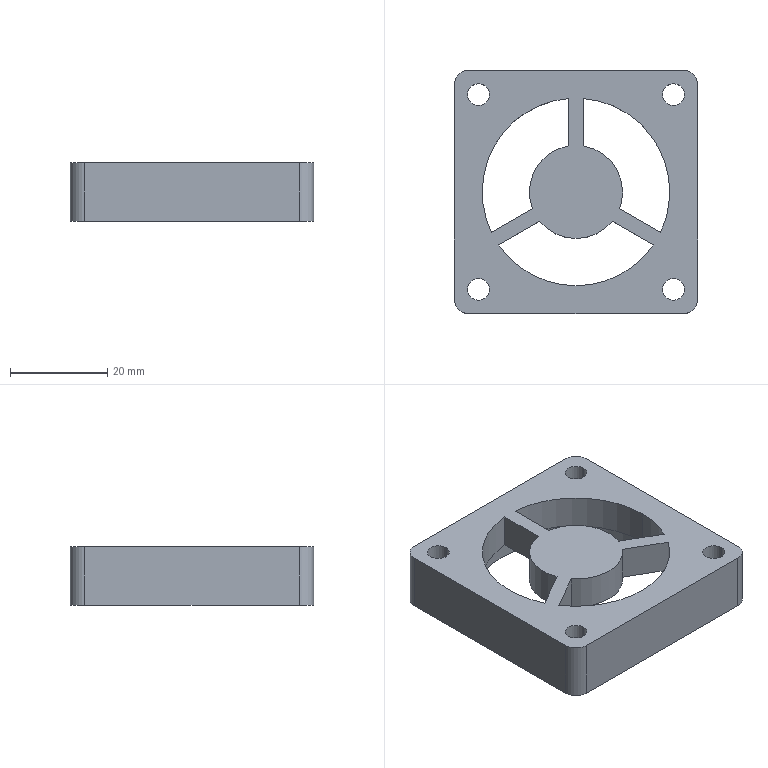Part | SolidWorks | features ICE 2, Extrusion 1 | 1 solid | 35 faces | box 50 x 50 x 12 mm | volume 16391 mm3 | cylinder 22 | plane 13 | commonest cylinder face diameters 4.5 x8 6 x4 19.118 x4 38.495 x4 42.899 x2
STEP:
#1=CARTESIAN_POINT('',(21.45,0.,5.));
#2=VERTEX_POINT('',#1);
#3=CARTESIAN_POINT('',(-21.45,0.,5.));
#4=VERTEX_POINT('',#3);
#5=CARTESIAN_POINT('',(0.,0.,5.));
#6=DIRECTION('',(0.,0.,-1.));
#7=DIRECTION('',(-1.,0.,0.));
#8=AXIS2_PLACEMENT_3D('',#5,#6,#7);
#9=CIRCLE('',#8,21.45);
#10=EDGE_CURVE('',#2,#4,#9,.T.);
#11=ORIENTED_EDGE('',*,*,#10,.F.);
#12=CARTESIAN_POINT('',(21.45,0.,0.));
#13=VERTEX_POINT('',#12);
#14=CARTESIAN_POINT('',(21.45,0.,5.));
#15=DIRECTION('',(0.,0.,-1.));
#16=VECTOR('',#15,1000.);
#17=LINE('',#14,#16);
#18=EDGE_CURVE('',#2,#13,#17,.T.);
#19=ORIENTED_EDGE('',*,*,#18,.T.);
#20=CARTESIAN_POINT('',(-21.45,0.,0.));
#21=VERTEX_POINT('',#20);
#22=CARTESIAN_POINT('',(0.,0.,0.));
#23=DIRECTION('',(0.,0.,-1.));
#24=DIRECTION('',(-1.,0.,0.));
#25=AXIS2_PLACEMENT_3D('',#22,#23,#24);
#26=CIRCLE('',#25,21.45);
#27=EDGE_CURVE('',#13,#21,#26,.T.);
#28=ORIENTED_EDGE('',*,*,#27,.T.);
#29=CARTESIAN_POINT('',(-21.45,0.,5.));
#30=DIRECTION('',(0.,0.,-1.));
#31=VECTOR('',#30,1000.);
#32=LINE('',#29,#31);
#33=EDGE_CURVE('',#4,#21,#32,.T.);
#34=ORIENTED_EDGE('',*,*,#33,.F.);
#35=EDGE_LOOP('',(#11,#19,#28,#34));
#36=FACE_OUTER_BOUND('',#35,.T.);
#37=CARTESIAN_POINT('',(0.,0.,5.));
#38=DIRECTION('',(0.,0.,-1.));
#39=DIRECTION('',(-1.,0.,0.));
#40=AXIS2_PLACEMENT_3D('',#37,#38,#39);
#41=CYLINDRICAL_SURFACE('',#40,21.45);
#42=ADVANCED_FACE('',(#36),#41,.F.);
#43=CARTESIAN_POINT('',(-22.25,-20.,12.));
#44=VERTEX_POINT('',#43);
#45=CARTESIAN_POINT('',(-17.75,-20.,12.));
#46=VERTEX_POINT('',#45);
#47=CARTESIAN_POINT('',(-20.,-20.,12.));
#48=DIRECTION('',(0.,0.,1.));
#49=DIRECTION('',(1.,0.,0.));
#50=AXIS2_PLACEMENT_3D('',#47,#48,#49);
#51=CIRCLE('',#50,2.25);
#52=EDGE_CURVE('',#44,#46,#51,.T.);
#53=ORIENTED_EDGE('',*,*,#52,.T.);
#54=CARTESIAN_POINT('',(-17.75,-20.,0.));
#55=VERTEX_POINT('',#54);
#56=CARTESIAN_POINT('',(-17.75,-20.,12.));
#57=DIRECTION('',(0.,0.,-1.));
#58=VECTOR('',#57,1000.);
#59=LINE('',#56,#58);
#60=EDGE_CURVE('',#46,#55,#59,.T.);
#61=ORIENTED_EDGE('',*,*,#60,.T.);
#62=CARTESIAN_POINT('',(-22.25,-20.,0.));
#63=VERTEX_POINT('',#62);
#64=CARTESIAN_POINT('',(-20.,-20.,0.));
#65=DIRECTION('',(0.,0.,1.));
#66=DIRECTION('',(1.,0.,0.));
#67=AXIS2_PLACEMENT_3D('',#64,#65,#66);
#68=CIRCLE('',#67,2.25);
#69=EDGE_CURVE('',#63,#55,#68,.T.);
#70=ORIENTED_EDGE('',*,*,#69,.F.);
#71=CARTESIAN_POINT('',(-22.25,-20.,12.));
#72=DIRECTION('',(0.,0.,-1.));
#73=VECTOR('',#72,1000.);
#74=LINE('',#71,#73);
#75=EDGE_CURVE('',#44,#63,#74,.T.);
#76=ORIENTED_EDGE('',*,*,#75,.F.);
#77=EDGE_LOOP('',(#53,#61,#70,#76));
#78=FACE_OUTER_BOUND('',#77,.T.);
#79=CARTESIAN_POINT('',(-20.,-20.,12.));
#80=DIRECTION('',(0.,0.,-1.));
#81=DIRECTION('',(-1.,0.,0.));
#82=AXIS2_PLACEMENT_3D('',#79,#80,#81);
#83=CYLINDRICAL_SURFACE('',#82,2.25);
#84=ADVANCED_FACE('',(#78),#83,.F.);
#85=CARTESIAN_POINT('',(17.75,-20.,12.));
#86=VERTEX_POINT('',#85);
#87=CARTESIAN_POINT('',(22.25,-20.,12.));
#88=VERTEX_POINT('',#87);
#89=CARTESIAN_POINT('',(20.,-20.,12.));
#90=DIRECTION('',(0.,0.,1.));
#91=DIRECTION('',(1.,0.,0.));
#92=AXIS2_PLACEMENT_3D('',#89,#90,#91);
#93=CIRCLE('',#92,2.25);
#94=EDGE_CURVE('',#86,#88,#93,.T.);
#95=ORIENTED_EDGE('',*,*,#94,.T.);
#96=CARTESIAN_POINT('',(22.25,-20.,0.));
#97=VERTEX_POINT('',#96);
#98=CARTESIAN_POINT('',(22.25,-20.,12.));
#99=DIRECTION('',(0.,0.,-1.));
#100=VECTOR('',#99,1000.);
#101=LINE('',#98,#100);
#102=EDGE_CURVE('',#88,#97,#101,.T.);
#103=ORIENTED_EDGE('',*,*,#102,.T.);
#104=CARTESIAN_POINT('',(17.75,-20.,0.));
#105=VERTEX_POINT('',#104);
#106=CARTESIAN_POINT('',(20.,-20.,0.));
#107=DIRECTION('',(0.,0.,1.));
#108=DIRECTION('',(1.,0.,0.));
#109=AXIS2_PLACEMENT_3D('',#106,#107,#108);
#110=CIRCLE('',#109,2.25);
#111=EDGE_CURVE('',#105,#97,#110,.T.);
#112=ORIENTED_EDGE('',*,*,#111,.F.);
#113=CARTESIAN_POINT('',(17.75,-20.,12.));
#114=DIRECTION('',(0.,0.,-1.));
#115=VECTOR('',#114,1000.);
#116=LINE('',#113,#115);
#117=EDGE_CURVE('',#86,#105,#116,.T.);
#118=ORIENTED_EDGE('',*,*,#117,.F.);
#119=EDGE_LOOP('',(#95,#103,#112,#118));
#120=FACE_OUTER_BOUND('',#119,.T.);
#121=CARTESIAN_POINT('',(20.,-20.,12.));
#122=DIRECTION('',(0.,0.,-1.));
#123=DIRECTION('',(-1.,0.,0.));
#124=AXIS2_PLACEMENT_3D('',#121,#122,#123);
#125=CYLINDRICAL_SURFACE('',#124,2.25);
#126=ADVANCED_FACE('',(#120),#125,.F.);
#127=CARTESIAN_POINT('',(17.75,20.,12.));
#128=VERTEX_POINT('',#127);
#129=CARTESIAN_POINT('',(22.25,20.,12.));
#130=VERTEX_POINT('',#129);
#131=CARTESIAN_POINT('',(20.,20.,12.));
#132=DIRECTION('',(0.,0.,1.));
#133=DIRECTION('',(1.,0.,0.));
#134=AXIS2_PLACEMENT_3D('',#131,#132,#133);
#135=CIRCLE('',#134,2.25);
#136=EDGE_CURVE('',#128,#130,#135,.T.);
#137=ORIENTED_EDGE('',*,*,#136,.T.);
#138=CARTESIAN_POINT('',(22.25,20.,0.));
#139=VERTEX_POINT('',#138);
#140=CARTESIAN_POINT('',(22.25,20.,12.));
#141=DIRECTION('',(0.,0.,-1.));
#142=VECTOR('',#141,1000.);
#143=LINE('',#140,#142);
#144=EDGE_CURVE('',#130,#139,#143,.T.);
#145=ORIENTED_EDGE('',*,*,#144,.T.);
#146=CARTESIAN_POINT('',(17.75,20.,0.));
#147=VERTEX_POINT('',#146);
#148=CARTESIAN_POINT('',(20.,20.,0.));
#149=DIRECTION('',(0.,0.,1.));
#150=DIRECTION('',(1.,0.,0.));
#151=AXIS2_PLACEMENT_3D('',#148,#149,#150);
#152=CIRCLE('',#151,2.25);
#153=EDGE_CURVE('',#147,#139,#152,.T.);
#154=ORIENTED_EDGE('',*,*,#153,.F.);
#155=CARTESIAN_POINT('',(17.75,20.,12.));
#156=DIRECTION('',(0.,0.,-1.));
#157=VECTOR('',#156,1000.);
#158=LINE('',#155,#157);
#159=EDGE_CURVE('',#128,#147,#158,.T.);
#160=ORIENTED_EDGE('',*,*,#159,.F.);
#161=EDGE_LOOP('',(#137,#145,#154,#160));
#162=FACE_OUTER_BOUND('',#161,.T.);
#163=CARTESIAN_POINT('',(20.,20.,12.));
#164=DIRECTION('',(0.,0.,-1.));
#165=DIRECTION('',(-1.,0.,0.));
#166=AXIS2_PLACEMENT_3D('',#163,#164,#165);
#167=CYLINDRICAL_SURFACE('',#166,2.25);
#168=ADVANCED_FACE('',(#162),#167,.F.);
#169=CARTESIAN_POINT('',(-22.25,20.,12.));
#170=VERTEX_POINT('',#169);
#171=CARTESIAN_POINT('',(-17.75,20.,12.));
#172=VERTEX_POINT('',#171);
#173=CARTESIAN_POINT('',(-20.,20.,12.));
#174=DIRECTION('',(0.,0.,1.));
#175=DIRECTION('',(1.,0.,0.));
#176=AXIS2_PLACEMENT_3D('',#173,#174,#175);
#177=CIRCLE('',#176,2.25);
#178=EDGE_CURVE('',#170,#172,#177,.T.);
#179=ORIENTED_EDGE('',*,*,#178,.T.);
#180=CARTESIAN_POINT('',(-17.75,20.,0.));
#181=VERTEX_POINT('',#180);
#182=CARTESIAN_POINT('',(-17.75,20.,12.));
#183=DIRECTION('',(0.,0.,-1.));
#184=VECTOR('',#183,1000.);
#185=LINE('',#182,#184);
#186=EDGE_CURVE('',#172,#181,#185,.T.);
#187=ORIENTED_EDGE('',*,*,#186,.T.);
#188=CARTESIAN_POINT('',(-22.25,20.,0.));
#189=VERTEX_POINT('',#188);
#190=CARTESIAN_POINT('',(-20.,20.,0.));
#191=DIRECTION('',(0.,0.,1.));
#192=DIRECTION('',(1.,0.,0.));
#193=AXIS2_PLACEMENT_3D('',#190,#191,#192);
#194=CIRCLE('',#193,2.25);
#195=EDGE_CURVE('',#189,#181,#194,.T.);
#196=ORIENTED_EDGE('',*,*,#195,.F.);
#197=CARTESIAN_POINT('',(-22.25,20.,12.));
#198=DIRECTION('',(0.,0.,-1.));
#199=VECTOR('',#198,1000.);
#200=LINE('',#197,#199);
#201=EDGE_CURVE('',#170,#189,#200,.T.);
#202=ORIENTED_EDGE('',*,*,#201,.F.);
#203=EDGE_LOOP('',(#179,#187,#196,#202));
#204=FACE_OUTER_BOUND('',#203,.T.);
#205=CARTESIAN_POINT('',(-20.,20.,12.));
#206=DIRECTION('',(0.,0.,-1.));
#207=DIRECTION('',(-1.,0.,0.));
#208=AXIS2_PLACEMENT_3D('',#205,#206,#207);
#209=CYLINDRICAL_SURFACE('',#208,2.25);
#210=ADVANCED_FACE('',(#204),#209,.F.);
#211=CARTESIAN_POINT('',(9.559,0.,5.));
#212=VERTEX_POINT('',#211);
#213=CARTESIAN_POINT('',(8.926,-3.421,5.));
#214=VERTEX_POINT('',#213);
#215=CARTESIAN_POINT('',(0.,0.,5.));
#216=DIRECTION('',(0.,0.,-1.));
#217=DIRECTION('',(-1.,0.,0.));
#218=AXIS2_PLACEMENT_3D('',#215,#216,#217);
#219=CIRCLE('',#218,9.559);
#220=EDGE_CURVE('',#212,#214,#219,.T.);
#221=ORIENTED_EDGE('',*,*,#220,.F.);
#222=CARTESIAN_POINT('',(9.559,0.,12.));
#223=VERTEX_POINT('',#222);
#224=CARTESIAN_POINT('',(9.559,0.,0.));
#225=DIRECTION('',(0.,0.,1.));
#226=VECTOR('',#225,1000.);
#227=LINE('',#224,#226);
#228=EDGE_CURVE('',#212,#223,#227,.T.);
#229=ORIENTED_EDGE('',*,*,#228,.T.);
#230=CARTESIAN_POINT('',(8.926,-3.421,12.));
#231=VERTEX_POINT('',#230);
#232=CARTESIAN_POINT('',(0.,0.,12.));
#233=DIRECTION('',(0.,0.,-1.));
#234=DIRECTION('',(1.,0.,0.));
#235=AXIS2_PLACEMENT_3D('',#232,#233,#234);
#236=CIRCLE('',#235,9.559);
#237=EDGE_CURVE('',#223,#231,#236,.T.);
#238=ORIENTED_EDGE('',*,*,#237,.T.);
#239=CARTESIAN_POINT('',(8.926,-3.421,0.));
#240=DIRECTION('',(0.,0.,1.));
#241=VECTOR('',#240,1000.);
#242=LINE('',#239,#241);
#243=EDGE_CURVE('',#214,#231,#242,.T.);
#244=ORIENTED_EDGE('',*,*,#243,.F.);
#245=EDGE_LOOP('',(#221,#229,#238,#244));
#246=FACE_OUTER_BOUND('',#245,.T.);
#247=CARTESIAN_POINT('',(0.,0.,0.));
#248=DIRECTION('',(0.,0.,1.));
#249=DIRECTION('',(1.,0.,0.));
#250=AXIS2_PLACEMENT_3D('',#247,#248,#249);
#251=CYLINDRICAL_SURFACE('',#250,9.559);
#252=ADVANCED_FACE('',(#246),#251,.T.);
#253=CARTESIAN_POINT('',(19.247,0.,5.));
#254=VERTEX_POINT('',#253);
#255=CARTESIAN_POINT('',(1.5,19.189,5.));
#256=VERTEX_POINT('',#255);
#257=CARTESIAN_POINT('',(0.,0.,5.));
#258=DIRECTION('',(0.,0.,1.));
#259=DIRECTION('',(-1.,0.,0.));
#260=AXIS2_PLACEMENT_3D('',#257,#258,#259);
#261=CIRCLE('',#260,19.247);
#262=EDGE_CURVE('',#254,#256,#261,.T.);
#263=ORIENTED_EDGE('',*,*,#262,.F.);
#264=CARTESIAN_POINT('',(19.247,0.,12.));
#265=VERTEX_POINT('',#264);
#266=CARTESIAN_POINT('',(19.247,0.,0.));
#267=DIRECTION('',(0.,0.,1.));
#268=VECTOR('',#267,1000.);
#269=LINE('',#266,#268);
#270=EDGE_CURVE('',#254,#265,#269,.T.);
#271=ORIENTED_EDGE('',*,*,#270,.T.);
#272=CARTESIAN_POINT('',(1.5,19.189,12.));
#273=VERTEX_POINT('',#272);
#274=CARTESIAN_POINT('',(0.,0.,12.));
#275=DIRECTION('',(0.,0.,1.));
#276=DIRECTION('',(1.,0.,0.));
#277=AXIS2_PLACEMENT_3D('',#274,#275,#276);
#278=CIRCLE('',#277,19.247);
#279=EDGE_CURVE('',#265,#273,#278,.T.);
#280=ORIENTED_EDGE('',*,*,#279,.T.);
#281=CARTESIAN_POINT('',(1.5,19.189,0.));
#282=DIRECTION('',(0.,0.,1.));
#283=VECTOR('',#282,1000.);
#284=LINE('',#281,#283);
#285=EDGE_CURVE('',#256,#273,#284,.T.);
#286=ORIENTED_EDGE('',*,*,#285,.F.);
#287=EDGE_LOOP('',(#263,#271,#280,#286));
#288=FACE_OUTER_BOUND('',#287,.T.);
#289=CARTESIAN_POINT('',(0.,0.,0.));
#290=DIRECTION('',(0.,0.,1.));
#291=DIRECTION('',(1.,0.,0.));
#292=AXIS2_PLACEMENT_3D('',#289,#290,#291);
#293=CYLINDRICAL_SURFACE('',#292,19.247);
#294=ADVANCED_FACE('',(#288),#293,.F.);
#295=ORIENTED_EDGE('',*,*,#270,.F.);
#296=CARTESIAN_POINT('',(17.368,-8.295,5.));
#297=VERTEX_POINT('',#296);
#298=CARTESIAN_POINT('',(0.,0.,5.));
#299=DIRECTION('',(0.,0.,1.));
#300=DIRECTION('',(-1.,0.,0.));
#301=AXIS2_PLACEMENT_3D('',#298,#299,#300);
#302=CIRCLE('',#301,19.247);
#303=EDGE_CURVE('',#297,#254,#302,.T.);
#304=ORIENTED_EDGE('',*,*,#303,.F.);
#305=CARTESIAN_POINT('',(17.368,-8.295,12.));
#306=VERTEX_POINT('',#305);
#307=CARTESIAN_POINT('',(17.368,-8.295,0.));
#308=DIRECTION('',(0.,0.,1.));
#309=VECTOR('',#308,1000.);
#310=LINE('',#307,#309);
#311=EDGE_CURVE('',#297,#306,#310,.T.);
#312=ORIENTED_EDGE('',*,*,#311,.T.);
#313=CARTESIAN_POINT('',(0.,0.,12.));
#314=DIRECTION('',(0.,0.,1.));
#315=DIRECTION('',(1.,0.,0.));
#316=AXIS2_PLACEMENT_3D('',#313,#314,#315);
#317=CIRCLE('',#316,19.247);
#318=EDGE_CURVE('',#306,#265,#317,.T.);
#319=ORIENTED_EDGE('',*,*,#318,.T.);
#320=EDGE_LOOP('',(#295,#304,#312,#319));
#321=FACE_OUTER_BOUND('',#320,.T.);
#322=CARTESIAN_POINT('',(0.,0.,0.));
#323=DIRECTION('',(0.,0.,1.));
#324=DIRECTION('',(1.,0.,0.));
#325=AXIS2_PLACEMENT_3D('',#322,#323,#324);
#326=CYLINDRICAL_SURFACE('',#325,19.247);
#327=ADVANCED_FACE('',(#321),#326,.F.);
#328=CARTESIAN_POINT('',(17.368,-8.295,5.));
#329=DIRECTION('',(0.866,-0.5,0.));
#330=VECTOR('',#329,1000.);
#331=LINE('',#328,#330);
#332=EDGE_CURVE('',#214,#297,#331,.T.);
#333=ORIENTED_EDGE('',*,*,#332,.F.);
#334=ORIENTED_EDGE('',*,*,#243,.T.);
#335=CARTESIAN_POINT('',(17.368,-8.295,12.));
#336=DIRECTION('',(0.866,-0.5,0.));
#337=VECTOR('',#336,1000.);
#338=LINE('',#335,#337);
#339=EDGE_CURVE('',#231,#306,#338,.T.);
#340=ORIENTED_EDGE('',*,*,#339,.T.);
#341=ORIENTED_EDGE('',*,*,#311,.F.);
#342=EDGE_LOOP('',(#333,#334,#340,#341));
#343=FACE_OUTER_BOUND('',#342,.T.);
#344=CARTESIAN_POINT('',(17.368,-8.295,0.));
#345=DIRECTION('',(-0.5,-0.866,0.));
#346=DIRECTION('',(0.866,-0.5,0.));
#347=AXIS2_PLACEMENT_3D('',#344,#345,#346);
#348=PLANE('',#347);
#349=ADVANCED_FACE('',(#343),#348,.F.);
#350=ORIENTED_EDGE('',*,*,#228,.F.);
#351=CARTESIAN_POINT('',(1.5,9.441,5.));
#352=VERTEX_POINT('',#351);
#353=CARTESIAN_POINT('',(0.,0.,5.));
#354=DIRECTION('',(0.,0.,-1.));
#355=DIRECTION('',(-1.,0.,0.));
#356=AXIS2_PLACEMENT_3D('',#353,#354,#355);
#357=CIRCLE('',#356,9.559);
#358=EDGE_CURVE('',#352,#212,#357,.T.);
#359=ORIENTED_EDGE('',*,*,#358,.F.);
#360=CARTESIAN_POINT('',(1.5,9.441,12.));
#361=VERTEX_POINT('',#360);
#362=CARTESIAN_POINT('',(1.5,9.441,0.));
#363=DIRECTION('',(0.,0.,1.));
#364=VECTOR('',#363,1000.);
#365=LINE('',#362,#364);
#366=EDGE_CURVE('',#352,#361,#365,.T.);
#367=ORIENTED_EDGE('',*,*,#366,.T.);
#368=CARTESIAN_POINT('',(0.,0.,12.));
#369=DIRECTION('',(0.,0.,-1.));
#370=DIRECTION('',(1.,0.,0.));
#371=AXIS2_PLACEMENT_3D('',#368,#369,#370);
#372=CIRCLE('',#371,9.559);
#373=EDGE_CURVE('',#361,#223,#372,.T.);
#374=ORIENTED_EDGE('',*,*,#373,.T.);
#375=EDGE_LOOP('',(#350,#359,#367,#374));
#376=FACE_OUTER_BOUND('',#375,.T.);
#377=CARTESIAN_POINT('',(0.,0.,0.));
#378=DIRECTION('',(0.,0.,1.));
#379=DIRECTION('',(1.,0.,0.));
#380=AXIS2_PLACEMENT_3D('',#377,#378,#379);
#381=CYLINDRICAL_SURFACE('',#380,9.559);
#382=ADVANCED_FACE('',(#376),#381,.T.);
#383=CARTESIAN_POINT('',(1.5,19.189,5.));
#384=DIRECTION('',(0.,-1.,0.));
#385=VECTOR('',#384,1000.);
#386=LINE('',#383,#385);
#387=EDGE_CURVE('',#256,#352,#386,.T.);
#388=ORIENTED_EDGE('',*,*,#387,.F.);
#389=ORIENTED_EDGE('',*,*,#285,.T.);
#390=CARTESIAN_POINT('',(1.5,19.189,12.));
#391=DIRECTION('',(0.,-1.,0.));
#392=VECTOR('',#391,1000.);
#393=LINE('',#390,#392);
#394=EDGE_CURVE('',#273,#361,#393,.T.);
#395=ORIENTED_EDGE('',*,*,#394,.T.);
#396=ORIENTED_EDGE('',*,*,#366,.F.);
#397=EDGE_LOOP('',(#388,#389,#395,#396));
#398=FACE_OUTER_BOUND('',#397,.T.);
#399=CARTESIAN_POINT('',(1.5,19.189,0.));
#400=DIRECTION('',(-1.,0.,0.));
#401=DIRECTION('',(0.,-1.,0.));
#402=AXIS2_PLACEMENT_3D('',#399,#400,#401);
#403=PLANE('',#402);
#404=ADVANCED_FACE('',(#398),#403,.F.);
#405=CARTESIAN_POINT('',(-15.868,-10.893,5.));
#406=VERTEX_POINT('',#405);
#407=CARTESIAN_POINT('',(15.868,-10.893,5.));
#408=VERTEX_POINT('',#407);
#409=CARTESIAN_POINT('',(0.,0.,5.));
#410=DIRECTION('',(0.,0.,1.));
#411=DIRECTION('',(-1.,0.,0.));
#412=AXIS2_PLACEMENT_3D('',#409,#410,#411);
#413=CIRCLE('',#412,19.247);
#414=EDGE_CURVE('',#406,#408,#413,.T.);
#415=ORIENTED_EDGE('',*,*,#414,.F.);
#416=CARTESIAN_POINT('',(-15.868,-10.893,12.));
#417=VERTEX_POINT('',#416);
#418=CARTESIAN_POINT('',(-15.868,-10.893,0.));
#419=DIRECTION('',(0.,0.,1.));
#420=VECTOR('',#419,1000.);
#421=LINE('',#418,#420);
#422=EDGE_CURVE('',#406,#417,#421,.T.);
#423=ORIENTED_EDGE('',*,*,#422,.T.);
#424=CARTESIAN_POINT('',(15.868,-10.893,12.));
#425=VERTEX_POINT('',#424);
#426=CARTESIAN_POINT('',(0.,0.,12.));
#427=DIRECTION('',(0.,0.,1.));
#428=DIRECTION('',(1.,0.,0.));
#429=AXIS2_PLACEMENT_3D('',#426,#427,#428);
#430=CIRCLE('',#429,19.247);
#431=EDGE_CURVE('',#417,#425,#430,.T.);
#432=ORIENTED_EDGE('',*,*,#431,.T.);
#433=CARTESIAN_POINT('',(15.868,-10.893,0.));
#434=DIRECTION('',(0.,0.,1.));
#435=VECTOR('',#434,1000.);
#436=LINE('',#433,#435);
#437=EDGE_CURVE('',#408,#425,#436,.T.);
#438=ORIENTED_EDGE('',*,*,#437,.F.);
#439=EDGE_LOOP('',(#415,#423,#432,#438));
#440=FACE_OUTER_BOUND('',#439,.T.);
#441=CARTESIAN_POINT('',(0.,0.,0.));
#442=DIRECTION('',(0.,0.,1.));
#443=DIRECTION('',(1.,0.,0.));
#444=AXIS2_PLACEMENT_3D('',#441,#442,#443);
#445=CYLINDRICAL_SURFACE('',#444,19.247);
#446=ADVANCED_FACE('',(#440),#445,.F.);
#447=CARTESIAN_POINT('',(-7.426,-6.019,5.));
#448=VERTEX_POINT('',#447);
#449=CARTESIAN_POINT('',(-15.868,-10.893,5.));
#450=DIRECTION('',(-0.866,-0.5,0.));
#451=VECTOR('',#450,1000.);
#452=LINE('',#449,#451);
#453=EDGE_CURVE('',#448,#406,#452,.T.);
#454=ORIENTED_EDGE('',*,*,#453,.F.);
#455=CARTESIAN_POINT('',(-7.426,-6.019,12.));
#456=VERTEX_POINT('',#455);
#457=CARTESIAN_POINT('',(-7.426,-6.019,0.));
#458=DIRECTION('',(0.,0.,1.));
#459=VECTOR('',#458,1000.);
#460=LINE('',#457,#459);
#461=EDGE_CURVE('',#448,#456,#460,.T.);
#462=ORIENTED_EDGE('',*,*,#461,.T.);
#463=CARTESIAN_POINT('',(-15.868,-10.893,12.));
#464=DIRECTION('',(-0.866,-0.5,0.));
#465=VECTOR('',#464,1000.);
#466=LINE('',#463,#465);
#467=EDGE_CURVE('',#456,#417,#466,.T.);
#468=ORIENTED_EDGE('',*,*,#467,.T.);
#469=ORIENTED_EDGE('',*,*,#422,.F.);
#470=EDGE_LOOP('',(#454,#462,#468,#469));
#471=FACE_OUTER_BOUND('',#470,.T.);
#472=CARTESIAN_POINT('',(-15.868,-10.893,0.));
#473=DIRECTION('',(-0.5,0.866,0.));
#474=DIRECTION('',(-0.866,-0.5,0.));
#475=AXIS2_PLACEMENT_3D('',#472,#473,#474);
#476=PLANE('',#475);
#477=ADVANCED_FACE('',(#471),#476,.F.);
#478=CARTESIAN_POINT('',(7.426,-6.019,5.));
#479=VERTEX_POINT('',#478);
#480=CARTESIAN_POINT('',(0.,0.,5.));
#481=DIRECTION('',(0.,0.,-1.));
#482=DIRECTION('',(-1.,0.,0.));
#483=AXIS2_PLACEMENT_3D('',#480,#481,#482);
#484=CIRCLE('',#483,9.559);
#485=EDGE_CURVE('',#479,#448,#484,.T.);
#486=ORIENTED_EDGE('',*,*,#485,.F.);
#487=CARTESIAN_POINT('',(7.426,-6.019,12.));
#488=VERTEX_POINT('',#487);
#489=CARTESIAN_POINT('',(7.426,-6.019,0.));
#490=DIRECTION('',(0.,0.,1.));
#491=VECTOR('',#490,1000.);
#492=LINE('',#489,#491);
#493=EDGE_CURVE('',#479,#488,#492,.T.);
#494=ORIENTED_EDGE('',*,*,#493,.T.);
#495=CARTESIAN_POINT('',(0.,0.,12.));
#496=DIRECTION('',(0.,0.,-1.));
#497=DIRECTION('',(1.,0.,0.));
#498=AXIS2_PLACEMENT_3D('',#495,#496,#497);
#499=CIRCLE('',#498,9.559);
#500=EDGE_CURVE('',#488,#456,#499,.T.);
#501=ORIENTED_EDGE('',*,*,#500,.T.);
#502=ORIENTED_EDGE('',*,*,#461,.F.);
#503=EDGE_LOOP('',(#486,#494,#501,#502));
#504=FACE_OUTER_BOUND('',#503,.T.);
#505=CARTESIAN_POINT('',(0.,0.,0.));
#506=DIRECTION('',(0.,0.,1.));
#507=DIRECTION('',(1.,0.,0.));
#508=AXIS2_PLACEMENT_3D('',#505,#506,#507);
#509=CYLINDRICAL_SURFACE('',#508,9.559);
#510=ADVANCED_FACE('',(#504),#509,.T.);
#511=CARTESIAN_POINT('',(15.868,-10.893,5.));
#512=DIRECTION('',(-0.866,0.5,0.));
#513=VECTOR('',#512,1000.);
#514=LINE('',#511,#513);
#515=EDGE_CURVE('',#408,#479,#514,.T.);
#516=ORIENTED_EDGE('',*,*,#515,.F.);
#517=ORIENTED_EDGE('',*,*,#437,.T.);
#518=CARTESIAN_POINT('',(15.868,-10.893,12.));
#519=DIRECTION('',(-0.866,0.5,0.));
#520=VECTOR('',#519,1000.);
#521=LINE('',#518,#520);
#522=EDGE_CURVE('',#425,#488,#521,.T.);
#523=ORIENTED_EDGE('',*,*,#522,.T.);
#524=ORIENTED_EDGE('',*,*,#493,.F.);
#525=EDGE_LOOP('',(#516,#517,#523,#524));
#526=FACE_OUTER_BOUND('',#525,.T.);
#527=CARTESIAN_POINT('',(15.868,-10.893,0.));
#528=DIRECTION('',(0.5,0.866,0.));
#529=DIRECTION('',(-0.866,0.5,0.));
#530=AXIS2_PLACEMENT_3D('',#527,#528,#529);
#531=PLANE('',#530);
#532=ADVANCED_FACE('',(#526),#531,.F.);
#533=CARTESIAN_POINT('',(-1.5,19.189,5.));
#534=VERTEX_POINT('',#533);
#535=CARTESIAN_POINT('',(-17.368,-8.295,5.));
#536=VERTEX_POINT('',#535);
#537=CARTESIAN_POINT('',(0.,0.,5.));
#538=DIRECTION('',(0.,0.,1.));
#539=DIRECTION('',(-1.,0.,0.));
#540=AXIS2_PLACEMENT_3D('',#537,#538,#539);
#541=CIRCLE('',#540,19.247);
#542=EDGE_CURVE('',#534,#536,#541,.T.);
#543=ORIENTED_EDGE('',*,*,#542,.F.);
#544=CARTESIAN_POINT('',(-1.5,19.189,12.));
#545=VERTEX_POINT('',#544);
#546=CARTESIAN_POINT('',(-1.5,19.189,0.));
#547=DIRECTION('',(0.,0.,1.));
#548=VECTOR('',#547,1000.);
#549=LINE('',#546,#548);
#550=EDGE_CURVE('',#534,#545,#549,.T.);
#551=ORIENTED_EDGE('',*,*,#550,.T.);
#552=CARTESIAN_POINT('',(-17.368,-8.295,12.));
#553=VERTEX_POINT('',#552);
#554=CARTESIAN_POINT('',(0.,0.,12.));
#555=DIRECTION('',(0.,0.,1.));
#556=DIRECTION('',(1.,0.,0.));
#557=AXIS2_PLACEMENT_3D('',#554,#555,#556);
#558=CIRCLE('',#557,19.247);
#559=EDGE_CURVE('',#545,#553,#558,.T.);
#560=ORIENTED_EDGE('',*,*,#559,.T.);
#561=CARTESIAN_POINT('',(-17.368,-8.295,0.));
#562=DIRECTION('',(0.,0.,1.));
#563=VECTOR('',#562,1000.);
#564=LINE('',#561,#563);
#565=EDGE_CURVE('',#536,#553,#564,.T.);
#566=ORIENTED_EDGE('',*,*,#565,.F.);
#567=EDGE_LOOP('',(#543,#551,#560,#566));
#568=FACE_OUTER_BOUND('',#567,.T.);
#569=CARTESIAN_POINT('',(0.,0.,0.));
#570=DIRECTION('',(0.,0.,1.));
#571=DIRECTION('',(1.,0.,0.));
#572=AXIS2_PLACEMENT_3D('',#569,#570,#571);
#573=CYLINDRICAL_SURFACE('',#572,19.247);
#574=ADVANCED_FACE('',(#568),#573,.F.);
#575=CARTESIAN_POINT('',(-1.5,9.441,5.));
#576=VERTEX_POINT('',#575);
#577=CARTESIAN_POINT('',(-1.5,19.189,5.));
#578=DIRECTION('',(0.,1.,0.));
#579=VECTOR('',#578,1000.);
#580=LINE('',#577,#579);
#581=EDGE_CURVE('',#576,#534,#580,.T.);
#582=ORIENTED_EDGE('',*,*,#581,.F.);
#583=CARTESIAN_POINT('',(-1.5,9.441,12.));
#584=VERTEX_POINT('',#583);
#585=CARTESIAN_POINT('',(-1.5,9.441,0.));
#586=DIRECTION('',(0.,0.,1.));
#587=VECTOR('',#586,1000.);
#588=LINE('',#585,#587);
#589=EDGE_CURVE('',#576,#584,#588,.T.);
#590=ORIENTED_EDGE('',*,*,#589,.T.);
#591=CARTESIAN_POINT('',(-1.5,19.189,12.));
#592=DIRECTION('',(0.,1.,0.));
#593=VECTOR('',#592,1000.);
#594=LINE('',#591,#593);
#595=EDGE_CURVE('',#584,#545,#594,.T.);
#596=ORIENTED_EDGE('',*,*,#595,.T.);
#597=ORIENTED_EDGE('',*,*,#550,.F.);
#598=EDGE_LOOP('',(#582,#590,#596,#597));
#599=FACE_OUTER_BOUND('',#598,.T.);
#600=CARTESIAN_POINT('',(-1.5,19.189,0.));
#601=DIRECTION('',(1.,0.,0.));
#602=DIRECTION('',(0.,1.,0.));
#603=AXIS2_PLACEMENT_3D('',#600,#601,#602);
#604=PLANE('',#603);
#605=ADVANCED_FACE('',(#599),#604,.F.);
#606=CARTESIAN_POINT('',(-8.926,-3.421,5.));
#607=VERTEX_POINT('',#606);
#608=CARTESIAN_POINT('',(0.,0.,5.));
#609=DIRECTION('',(0.,0.,-1.));
#610=DIRECTION('',(-1.,0.,0.));
#611=AXIS2_PLACEMENT_3D('',#608,#609,#610);
#612=CIRCLE('',#611,9.559);
#613=EDGE_CURVE('',#607,#576,#612,.T.);
#614=ORIENTED_EDGE('',*,*,#613,.F.);
#615=CARTESIAN_POINT('',(-8.926,-3.421,12.));
#616=VERTEX_POINT('',#615);
#617=CARTESIAN_POINT('',(-8.926,-3.421,0.));
#618=DIRECTION('',(0.,0.,1.));
#619=VECTOR('',#618,1000.);
#620=LINE('',#617,#619);
#621=EDGE_CURVE('',#607,#616,#620,.T.);
#622=ORIENTED_EDGE('',*,*,#621,.T.);
#623=CARTESIAN_POINT('',(0.,0.,12.));
#624=DIRECTION('',(0.,0.,-1.));
#625=DIRECTION('',(1.,0.,0.));
#626=AXIS2_PLACEMENT_3D('',#623,#624,#625);
#627=CIRCLE('',#626,9.559);
#628=EDGE_CURVE('',#616,#584,#627,.T.);
#629=ORIENTED_EDGE('',*,*,#628,.T.);
#630=ORIENTED_EDGE('',*,*,#589,.F.);
#631=EDGE_LOOP('',(#614,#622,#629,#630));
#632=FACE_OUTER_BOUND('',#631,.T.);
#633=CARTESIAN_POINT('',(0.,0.,0.));
#634=DIRECTION('',(0.,0.,1.));
#635=DIRECTION('',(1.,0.,0.));
#636=AXIS2_PLACEMENT_3D('',#633,#634,#635);
#637=CYLINDRICAL_SURFACE('',#636,9.559);
#638=ADVANCED_FACE('',(#632),#637,.T.);
#639=CARTESIAN_POINT('',(-17.368,-8.295,5.));
#640=DIRECTION('',(0.866,0.5,0.));
#641=VECTOR('',#640,1000.);
#642=LINE('',#639,#641);
#643=EDGE_CURVE('',#536,#607,#642,.T.);
#644=ORIENTED_EDGE('',*,*,#643,.F.);
#645=ORIENTED_EDGE('',*,*,#565,.T.);
#646=CARTESIAN_POINT('',(-17.368,-8.295,12.));
#647=DIRECTION('',(0.866,0.5,0.));
#648=VECTOR('',#647,1000.);
#649=LINE('',#646,#648);
#650=EDGE_CURVE('',#553,#616,#649,.T.);
#651=ORIENTED_EDGE('',*,*,#650,.T.);
#652=ORIENTED_EDGE('',*,*,#621,.F.);
#653=EDGE_LOOP('',(#644,#645,#651,#652));
#654=FACE_OUTER_BOUND('',#653,.T.);
#655=CARTESIAN_POINT('',(-17.368,-8.295,0.));
#656=DIRECTION('',(0.5,-0.866,0.));
#657=DIRECTION('',(0.866,0.5,0.));
#658=AXIS2_PLACEMENT_3D('',#655,#656,#657);
#659=PLANE('',#658);
#660=ADVANCED_FACE('',(#654),#659,.F.);
#661=ORIENTED_EDGE('',*,*,#559,.F.);
#662=ORIENTED_EDGE('',*,*,#595,.F.);
#663=ORIENTED_EDGE('',*,*,#628,.F.);
#664=ORIENTED_EDGE('',*,*,#650,.F.);
#665=EDGE_LOOP('',(#661,#662,#663,#664));
#666=FACE_BOUND('',#665,.T.);
#667=ORIENTED_EDGE('',*,*,#431,.F.);
#668=ORIENTED_EDGE('',*,*,#467,.F.);
#669=ORIENTED_EDGE('',*,*,#500,.F.);
#670=ORIENTED_EDGE('',*,*,#522,.F.);
#671=EDGE_LOOP('',(#667,#668,#669,#670));
#672=FACE_BOUND('',#671,.T.);
#673=ORIENTED_EDGE('',*,*,#318,.F.);
#674=ORIENTED_EDGE('',*,*,#339,.F.);
#675=ORIENTED_EDGE('',*,*,#237,.F.);
#676=ORIENTED_EDGE('',*,*,#373,.F.);
#677=ORIENTED_EDGE('',*,*,#394,.F.);
#678=ORIENTED_EDGE('',*,*,#279,.F.);
#679=EDGE_LOOP('',(#673,#674,#675,#676,#677,#678));
#680=FACE_BOUND('',#679,.T.);
#681=ORIENTED_EDGE('',*,*,#94,.F.);
#682=CARTESIAN_POINT('',(20.,-20.,12.));
#683=DIRECTION('',(0.,0.,1.));
#684=DIRECTION('',(1.,0.,0.));
#685=AXIS2_PLACEMENT_3D('',#682,#683,#684);
#686=CIRCLE('',#685,2.25);
#687=EDGE_CURVE('',#88,#86,#686,.T.);
#688=ORIENTED_EDGE('',*,*,#687,.F.);
#689=EDGE_LOOP('',(#681,#688));
#690=FACE_BOUND('',#689,.T.);
#691=ORIENTED_EDGE('',*,*,#178,.F.);
#692=CARTESIAN_POINT('',(-20.,20.,12.));
#693=DIRECTION('',(0.,0.,1.));
#694=DIRECTION('',(1.,0.,0.));
#695=AXIS2_PLACEMENT_3D('',#692,#693,#694);
#696=CIRCLE('',#695,2.25);
#697=EDGE_CURVE('',#172,#170,#696,.T.);
#698=ORIENTED_EDGE('',*,*,#697,.F.);
#699=EDGE_LOOP('',(#691,#698));
#700=FACE_BOUND('',#699,.T.);
#701=CARTESIAN_POINT('',(22.,-25.,12.));
#702=VERTEX_POINT('',#701);
#703=CARTESIAN_POINT('',(25.,-22.,12.));
#704=VERTEX_POINT('',#703);
#705=CARTESIAN_POINT('',(22.,-22.,12.));
#706=DIRECTION('',(0.,0.,1.));
#707=DIRECTION('',(1.,0.,0.));
#708=AXIS2_PLACEMENT_3D('',#705,#706,#707);
#709=CIRCLE('',#708,3.);
#710=EDGE_CURVE('',#702,#704,#709,.T.);
#711=ORIENTED_EDGE('',*,*,#710,.T.);
#712=CARTESIAN_POINT('',(25.,22.,12.));
#713=VERTEX_POINT('',#712);
#714=CARTESIAN_POINT('',(25.,22.,12.));
#715=DIRECTION('',(0.,1.,0.));
#716=VECTOR('',#715,1000.);
#717=LINE('',#714,#716);
#718=EDGE_CURVE('',#704,#713,#717,.T.);
#719=ORIENTED_EDGE('',*,*,#718,.T.);
#720=CARTESIAN_POINT('',(22.,25.,12.));
#721=VERTEX_POINT('',#720);
#722=CARTESIAN_POINT('',(22.,22.,12.));
#723=DIRECTION('',(0.,0.,1.));
#724=DIRECTION('',(-1.,0.,0.));
#725=AXIS2_PLACEMENT_3D('',#722,#723,#724);
#726=CIRCLE('',#725,3.);
#727=EDGE_CURVE('',#713,#721,#726,.T.);
#728=ORIENTED_EDGE('',*,*,#727,.T.);
#729=CARTESIAN_POINT('',(-22.,25.,12.));
#730=VERTEX_POINT('',#729);
#731=CARTESIAN_POINT('',(-22.,25.,12.));
#732=DIRECTION('',(-1.,0.,0.));
#733=VECTOR('',#732,1000.);
#734=LINE('',#731,#733);
#735=EDGE_CURVE('',#721,#730,#734,.T.);
#736=ORIENTED_EDGE('',*,*,#735,.T.);
#737=CARTESIAN_POINT('',(-25.,22.,12.));
#738=VERTEX_POINT('',#737);
#739=CARTESIAN_POINT('',(-22.,22.,12.));
#740=DIRECTION('',(0.,0.,1.));
#741=DIRECTION('',(1.,0.,0.));
#742=AXIS2_PLACEMENT_3D('',#739,#740,#741);
#743=CIRCLE('',#742,3.);
#744=EDGE_CURVE('',#730,#738,#743,.T.);
#745=ORIENTED_EDGE('',*,*,#744,.T.);
#746=CARTESIAN_POINT('',(-25.,-22.,12.));
#747=VERTEX_POINT('',#746);
#748=CARTESIAN_POINT('',(-25.,22.,12.));
#749=DIRECTION('',(0.,-1.,0.));
#750=VECTOR('',#749,1000.);
#751=LINE('',#748,#750);
#752=EDGE_CURVE('',#738,#747,#751,.T.);
#753=ORIENTED_EDGE('',*,*,#752,.T.);
#754=CARTESIAN_POINT('',(-22.,-25.,12.));
#755=VERTEX_POINT('',#754);
#756=CARTESIAN_POINT('',(-22.,-22.,12.));
#757=DIRECTION('',(0.,0.,1.));
#758=DIRECTION('',(1.,0.,0.));
#759=AXIS2_PLACEMENT_3D('',#756,#757,#758);
#760=CIRCLE('',#759,3.);
#761=EDGE_CURVE('',#747,#755,#760,.T.);
#762=ORIENTED_EDGE('',*,*,#761,.T.);
#763=CARTESIAN_POINT('',(-22.,-25.,12.));
#764=DIRECTION('',(1.,0.,0.));
#765=VECTOR('',#764,1000.);
#766=LINE('',#763,#765);
#767=EDGE_CURVE('',#755,#702,#766,.T.);
#768=ORIENTED_EDGE('',*,*,#767,.T.);
#769=EDGE_LOOP('',(#711,#719,#728,#736,#745,#753,#762,#768));
#770=FACE_OUTER_BOUND('',#769,.T.);
#771=ORIENTED_EDGE('',*,*,#136,.F.);
#772=CARTESIAN_POINT('',(20.,20.,12.));
#773=DIRECTION('',(0.,0.,1.));
#774=DIRECTION('',(1.,0.,0.));
#775=AXIS2_PLACEMENT_3D('',#772,#773,#774);
#776=CIRCLE('',#775,2.25);
#777=EDGE_CURVE('',#130,#128,#776,.T.);
#778=ORIENTED_EDGE('',*,*,#777,.F.);
#779=EDGE_LOOP('',(#771,#778));
#780=FACE_BOUND('',#779,.T.);
#781=ORIENTED_EDGE('',*,*,#52,.F.);
#782=CARTESIAN_POINT('',(-20.,-20.,12.));
#783=DIRECTION('',(0.,0.,1.));
#784=DIRECTION('',(1.,0.,0.));
#785=AXIS2_PLACEMENT_3D('',#782,#783,#784);
#786=CIRCLE('',#785,2.25);
#787=EDGE_CURVE('',#46,#44,#786,.T.);
#788=ORIENTED_EDGE('',*,*,#787,.F.);
#789=EDGE_LOOP('',(#781,#788));
#790=FACE_BOUND('',#789,.T.);
#791=CARTESIAN_POINT('',(22.,-22.,12.));
#792=DIRECTION('',(0.,0.,1.));
#793=DIRECTION('',(1.,0.,0.));
#794=AXIS2_PLACEMENT_3D('',#791,#792,#793);
#795=PLANE('',#794);
#796=ADVANCED_FACE('',(#666,#672,#680,#690,#700,#770,#780,#790),#795,.T.);
#797=CARTESIAN_POINT('',(0.,0.,0.));
#798=DIRECTION('',(0.,0.,-1.));
#799=DIRECTION('',(-1.,0.,0.));
#800=AXIS2_PLACEMENT_3D('',#797,#798,#799);
#801=CIRCLE('',#800,21.45);
#802=EDGE_CURVE('',#21,#13,#801,.T.);
#803=ORIENTED_EDGE('',*,*,#802,.F.);
#804=ORIENTED_EDGE('',*,*,#27,.F.);
#805=EDGE_LOOP('',(#803,#804));
#806=FACE_BOUND('',#805,.T.);
#807=CARTESIAN_POINT('',(22.,-25.,0.));
#808=VERTEX_POINT('',#807);
#809=CARTESIAN_POINT('',(25.,-22.,0.));
#810=VERTEX_POINT('',#809);
#811=CARTESIAN_POINT('',(22.,-22.,0.));
#812=DIRECTION('',(0.,0.,1.));
#813=DIRECTION('',(1.,0.,0.));
#814=AXIS2_PLACEMENT_3D('',#811,#812,#813);
#815=CIRCLE('',#814,3.);
#816=EDGE_CURVE('',#808,#810,#815,.T.);
#817=ORIENTED_EDGE('',*,*,#816,.F.);
#818=CARTESIAN_POINT('',(-22.,-25.,0.));
#819=VERTEX_POINT('',#818);
#820=CARTESIAN_POINT('',(-22.,-25.,0.));
#821=DIRECTION('',(1.,0.,0.));
#822=VECTOR('',#821,1000.);
#823=LINE('',#820,#822);
#824=EDGE_CURVE('',#819,#808,#823,.T.);
#825=ORIENTED_EDGE('',*,*,#824,.F.);
#826=CARTESIAN_POINT('',(-25.,-22.,0.));
#827=VERTEX_POINT('',#826);
#828=CARTESIAN_POINT('',(-22.,-22.,0.));
#829=DIRECTION('',(0.,0.,1.));
#830=DIRECTION('',(1.,0.,0.));
#831=AXIS2_PLACEMENT_3D('',#828,#829,#830);
#832=CIRCLE('',#831,3.);
#833=EDGE_CURVE('',#827,#819,#832,.T.);
#834=ORIENTED_EDGE('',*,*,#833,.F.);
#835=CARTESIAN_POINT('',(-25.,22.,0.));
#836=VERTEX_POINT('',#835);
#837=CARTESIAN_POINT('',(-25.,22.,0.));
#838=DIRECTION('',(0.,-1.,0.));
#839=VECTOR('',#838,1000.);
#840=LINE('',#837,#839);
#841=EDGE_CURVE('',#836,#827,#840,.T.);
#842=ORIENTED_EDGE('',*,*,#841,.F.);
#843=CARTESIAN_POINT('',(-22.,25.,0.));
#844=VERTEX_POINT('',#843);
#845=CARTESIAN_POINT('',(-22.,22.,0.));
#846=DIRECTION('',(0.,0.,1.));
#847=DIRECTION('',(1.,0.,0.));
#848=AXIS2_PLACEMENT_3D('',#845,#846,#847);
#849=CIRCLE('',#848,3.);
#850=EDGE_CURVE('',#844,#836,#849,.T.);
#851=ORIENTED_EDGE('',*,*,#850,.F.);
#852=CARTESIAN_POINT('',(22.,25.,0.));
#853=VERTEX_POINT('',#852);
#854=CARTESIAN_POINT('',(-22.,25.,0.));
#855=DIRECTION('',(-1.,0.,0.));
#856=VECTOR('',#855,1000.);
#857=LINE('',#854,#856);
#858=EDGE_CURVE('',#853,#844,#857,.T.);
#859=ORIENTED_EDGE('',*,*,#858,.F.);
#860=CARTESIAN_POINT('',(25.,22.,0.));
#861=VERTEX_POINT('',#860);
#862=CARTESIAN_POINT('',(22.,22.,0.));
#863=DIRECTION('',(0.,0.,1.));
#864=DIRECTION('',(-1.,0.,0.));
#865=AXIS2_PLACEMENT_3D('',#862,#863,#864);
#866=CIRCLE('',#865,3.);
#867=EDGE_CURVE('',#861,#853,#866,.T.);
#868=ORIENTED_EDGE('',*,*,#867,.F.);
#869=CARTESIAN_POINT('',(25.,22.,0.));
#870=DIRECTION('',(0.,1.,0.));
#871=VECTOR('',#870,1000.);
#872=LINE('',#869,#871);
#873=EDGE_CURVE('',#810,#861,#872,.T.);
#874=ORIENTED_EDGE('',*,*,#873,.F.);
#875=EDGE_LOOP('',(#817,#825,#834,#842,#851,#859,#868,#874));
#876=FACE_OUTER_BOUND('',#875,.T.);
#877=ORIENTED_EDGE('',*,*,#195,.T.);
#878=CARTESIAN_POINT('',(-20.,20.,0.));
#879=DIRECTION('',(0.,0.,1.));
#880=DIRECTION('',(1.,0.,0.));
#881=AXIS2_PLACEMENT_3D('',#878,#879,#880);
#882=CIRCLE('',#881,2.25);
#883=EDGE_CURVE('',#181,#189,#882,.T.);
#884=ORIENTED_EDGE('',*,*,#883,.T.);
#885=EDGE_LOOP('',(#877,#884));
#886=FACE_BOUND('',#885,.T.);
#887=ORIENTED_EDGE('',*,*,#153,.T.);
#888=CARTESIAN_POINT('',(20.,20.,0.));
#889=DIRECTION('',(0.,0.,1.));
#890=DIRECTION('',(1.,0.,0.));
#891=AXIS2_PLACEMENT_3D('',#888,#889,#890);
#892=CIRCLE('',#891,2.25);
#893=EDGE_CURVE('',#139,#147,#892,.T.);
#894=ORIENTED_EDGE('',*,*,#893,.T.);
#895=EDGE_LOOP('',(#887,#894));
#896=FACE_BOUND('',#895,.T.);
#897=ORIENTED_EDGE('',*,*,#111,.T.);
#898=CARTESIAN_POINT('',(20.,-20.,0.));
#899=DIRECTION('',(0.,0.,1.));
#900=DIRECTION('',(1.,0.,0.));
#901=AXIS2_PLACEMENT_3D('',#898,#899,#900);
#902=CIRCLE('',#901,2.25);
#903=EDGE_CURVE('',#97,#105,#902,.T.);
#904=ORIENTED_EDGE('',*,*,#903,.T.);
#905=EDGE_LOOP('',(#897,#904));
#906=FACE_BOUND('',#905,.T.);
#907=ORIENTED_EDGE('',*,*,#69,.T.);
#908=CARTESIAN_POINT('',(-20.,-20.,0.));
#909=DIRECTION('',(0.,0.,1.));
#910=DIRECTION('',(1.,0.,0.));
#911=AXIS2_PLACEMENT_3D('',#908,#909,#910);
#912=CIRCLE('',#911,2.25);
#913=EDGE_CURVE('',#55,#63,#912,.T.);
#914=ORIENTED_EDGE('',*,*,#913,.T.);
#915=EDGE_LOOP('',(#907,#914));
#916=FACE_BOUND('',#915,.T.);
#917=CARTESIAN_POINT('',(22.,-22.,0.));
#918=DIRECTION('',(0.,0.,1.));
#919=DIRECTION('',(1.,0.,0.));
#920=AXIS2_PLACEMENT_3D('',#917,#918,#919);
#921=PLANE('',#920);
#922=ADVANCED_FACE('',(#806,#876,#886,#896,#906,#916),#921,.F.);
#923=ORIENTED_EDGE('',*,*,#816,.T.);
#924=CARTESIAN_POINT('',(25.,-22.,12.));
#925=DIRECTION('',(0.,0.,-1.));
#926=VECTOR('',#925,1000.);
#927=LINE('',#924,#926);
#928=EDGE_CURVE('',#704,#810,#927,.T.);
#929=ORIENTED_EDGE('',*,*,#928,.F.);
#930=ORIENTED_EDGE('',*,*,#710,.F.);
#931=CARTESIAN_POINT('',(22.,-25.,12.));
#932=DIRECTION('',(0.,0.,-1.));
#933=VECTOR('',#932,1000.);
#934=LINE('',#931,#933);
#935=EDGE_CURVE('',#702,#808,#934,.T.);
#936=ORIENTED_EDGE('',*,*,#935,.T.);
#937=EDGE_LOOP('',(#923,#929,#930,#936));
#938=FACE_OUTER_BOUND('',#937,.T.);
#939=CARTESIAN_POINT('',(22.,-22.,12.));
#940=DIRECTION('',(0.,0.,-1.));
#941=DIRECTION('',(-1.,0.,0.));
#942=AXIS2_PLACEMENT_3D('',#939,#940,#941);
#943=CYLINDRICAL_SURFACE('',#942,3.);
#944=ADVANCED_FACE('',(#938),#943,.T.);
#945=ORIENTED_EDGE('',*,*,#873,.T.);
#946=CARTESIAN_POINT('',(25.,22.,12.));
#947=DIRECTION('',(0.,0.,-1.));
#948=VECTOR('',#947,1000.);
#949=LINE('',#946,#948);
#950=EDGE_CURVE('',#713,#861,#949,.T.);
#951=ORIENTED_EDGE('',*,*,#950,.F.);
#952=ORIENTED_EDGE('',*,*,#718,.F.);
#953=ORIENTED_EDGE('',*,*,#928,.T.);
#954=EDGE_LOOP('',(#945,#951,#952,#953));
#955=FACE_OUTER_BOUND('',#954,.T.);
#956=CARTESIAN_POINT('',(25.,22.,12.));
#957=DIRECTION('',(-1.,0.,0.));
#958=DIRECTION('',(0.,-1.,0.));
#959=AXIS2_PLACEMENT_3D('',#956,#957,#958);
#960=PLANE('',#959);
#961=ADVANCED_FACE('',(#955),#960,.F.);
#962=ORIENTED_EDGE('',*,*,#867,.T.);
#963=CARTESIAN_POINT('',(22.,25.,12.));
#964=DIRECTION('',(0.,0.,-1.));
#965=VECTOR('',#964,1000.);
#966=LINE('',#963,#965);
#967=EDGE_CURVE('',#721,#853,#966,.T.);
#968=ORIENTED_EDGE('',*,*,#967,.F.);
#969=ORIENTED_EDGE('',*,*,#727,.F.);
#970=ORIENTED_EDGE('',*,*,#950,.T.);
#971=EDGE_LOOP('',(#962,#968,#969,#970));
#972=FACE_OUTER_BOUND('',#971,.T.);
#973=CARTESIAN_POINT('',(22.,22.,12.));
#974=DIRECTION('',(0.,0.,-1.));
#975=DIRECTION('',(-1.,0.,0.));
#976=AXIS2_PLACEMENT_3D('',#973,#974,#975);
#977=CYLINDRICAL_SURFACE('',#976,3.);
#978=ADVANCED_FACE('',(#972),#977,.T.);
#979=ORIENTED_EDGE('',*,*,#858,.T.);
#980=CARTESIAN_POINT('',(-22.,25.,12.));
#981=DIRECTION('',(0.,0.,-1.));
#982=VECTOR('',#981,1000.);
#983=LINE('',#980,#982);
#984=EDGE_CURVE('',#730,#844,#983,.T.);
#985=ORIENTED_EDGE('',*,*,#984,.F.);
#986=ORIENTED_EDGE('',*,*,#735,.F.);
#987=ORIENTED_EDGE('',*,*,#967,.T.);
#988=EDGE_LOOP('',(#979,#985,#986,#987));
#989=FACE_OUTER_BOUND('',#988,.T.);
#990=CARTESIAN_POINT('',(-22.,25.,12.));
#991=DIRECTION('',(0.,-1.,0.));
#992=DIRECTION('',(0.,0.,-1.));
#993=AXIS2_PLACEMENT_3D('',#990,#991,#992);
#994=PLANE('',#993);
#995=ADVANCED_FACE('',(#989),#994,.F.);
#996=ORIENTED_EDGE('',*,*,#850,.T.);
#997=CARTESIAN_POINT('',(-25.,22.,12.));
#998=DIRECTION('',(0.,0.,-1.));
#999=VECTOR('',#998,1000.);
#1000=LINE('',#997,#999);
#1001=EDGE_CURVE('',#738,#836,#1000,.T.);
#1002=ORIENTED_EDGE('',*,*,#1001,.F.);
#1003=ORIENTED_EDGE('',*,*,#744,.F.);
#1004=ORIENTED_EDGE('',*,*,#984,.T.);
#1005=EDGE_LOOP('',(#996,#1002,#1003,#1004));
#1006=FACE_OUTER_BOUND('',#1005,.T.);
#1007=CARTESIAN_POINT('',(-22.,22.,12.));
#1008=DIRECTION('',(0.,0.,-1.));
#1009=DIRECTION('',(-1.,0.,0.));
#1010=AXIS2_PLACEMENT_3D('',#1007,#1008,#1009);
#1011=CYLINDRICAL_SURFACE('',#1010,3.);
#1012=ADVANCED_FACE('',(#1006),#1011,.T.);
#1013=ORIENTED_EDGE('',*,*,#841,.T.);
#1014=CARTESIAN_POINT('',(-25.,-22.,12.));
#1015=DIRECTION('',(0.,0.,-1.));
#1016=VECTOR('',#1015,1000.);
#1017=LINE('',#1014,#1016);
#1018=EDGE_CURVE('',#747,#827,#1017,.T.);
#1019=ORIENTED_EDGE('',*,*,#1018,.F.);
#1020=ORIENTED_EDGE('',*,*,#752,.F.);
#1021=ORIENTED_EDGE('',*,*,#1001,.T.);
#1022=EDGE_LOOP('',(#1013,#1019,#1020,#1021));
#1023=FACE_OUTER_BOUND('',#1022,.T.);
#1024=CARTESIAN_POINT('',(-25.,22.,12.));
#1025=DIRECTION('',(1.,0.,0.));
#1026=DIRECTION('',(0.,1.,0.));
#1027=AXIS2_PLACEMENT_3D('',#1024,#1025,#1026);
#1028=PLANE('',#1027);
#1029=ADVANCED_FACE('',(#1023),#1028,.F.);
#1030=ORIENTED_EDGE('',*,*,#833,.T.);
#1031=CARTESIAN_POINT('',(-22.,-25.,12.));
#1032=DIRECTION('',(0.,0.,-1.));
#1033=VECTOR('',#1032,1000.);
#1034=LINE('',#1031,#1033);
#1035=EDGE_CURVE('',#755,#819,#1034,.T.);
#1036=ORIENTED_EDGE('',*,*,#1035,.F.);
#1037=ORIENTED_EDGE('',*,*,#761,.F.);
#1038=ORIENTED_EDGE('',*,*,#1018,.T.);
#1039=EDGE_LOOP('',(#1030,#1036,#1037,#1038));
#1040=FACE_OUTER_BOUND('',#1039,.T.);
#1041=CARTESIAN_POINT('',(-22.,-22.,12.));
#1042=DIRECTION('',(0.,0.,-1.));
#1043=DIRECTION('',(-1.,0.,0.));
#1044=AXIS2_PLACEMENT_3D('',#1041,#1042,#1043);
#1045=CYLINDRICAL_SURFACE('',#1044,3.);
#1046=ADVANCED_FACE('',(#1040),#1045,.T.);
#1047=ORIENTED_EDGE('',*,*,#824,.T.);
#1048=ORIENTED_EDGE('',*,*,#935,.F.);
#1049=ORIENTED_EDGE('',*,*,#767,.F.);
#1050=ORIENTED_EDGE('',*,*,#1035,.T.);
#1051=EDGE_LOOP('',(#1047,#1048,#1049,#1050));
#1052=FACE_OUTER_BOUND('',#1051,.T.);
#1053=CARTESIAN_POINT('',(-22.,-25.,12.));
#1054=DIRECTION('',(0.,1.,0.));
#1055=DIRECTION('',(0.,0.,1.));
#1056=AXIS2_PLACEMENT_3D('',#1053,#1054,#1055);
#1057=PLANE('',#1056);
#1058=ADVANCED_FACE('',(#1052),#1057,.F.);
#1059=ORIENTED_EDGE('',*,*,#186,.F.);
#1060=ORIENTED_EDGE('',*,*,#697,.T.);
#1061=ORIENTED_EDGE('',*,*,#201,.T.);
#1062=ORIENTED_EDGE('',*,*,#883,.F.);
#1063=EDGE_LOOP('',(#1059,#1060,#1061,#1062));
#1064=FACE_OUTER_BOUND('',#1063,.T.);
#1065=CARTESIAN_POINT('',(-20.,20.,12.));
#1066=DIRECTION('',(0.,0.,-1.));
#1067=DIRECTION('',(-1.,0.,0.));
#1068=AXIS2_PLACEMENT_3D('',#1065,#1066,#1067);
#1069=CYLINDRICAL_SURFACE('',#1068,2.25);
#1070=ADVANCED_FACE('',(#1064),#1069,.F.);
#1071=ORIENTED_EDGE('',*,*,#144,.F.);
#1072=ORIENTED_EDGE('',*,*,#777,.T.);
#1073=ORIENTED_EDGE('',*,*,#159,.T.);
#1074=ORIENTED_EDGE('',*,*,#893,.F.);
#1075=EDGE_LOOP('',(#1071,#1072,#1073,#1074));
#1076=FACE_OUTER_BOUND('',#1075,.T.);
#1077=CARTESIAN_POINT('',(20.,20.,12.));
#1078=DIRECTION('',(0.,0.,-1.));
#1079=DIRECTION('',(-1.,0.,0.));
#1080=AXIS2_PLACEMENT_3D('',#1077,#1078,#1079);
#1081=CYLINDRICAL_SURFACE('',#1080,2.25);
#1082=ADVANCED_FACE('',(#1076),#1081,.F.);
#1083=ORIENTED_EDGE('',*,*,#102,.F.);
#1084=ORIENTED_EDGE('',*,*,#687,.T.);
#1085=ORIENTED_EDGE('',*,*,#117,.T.);
#1086=ORIENTED_EDGE('',*,*,#903,.F.);
#1087=EDGE_LOOP('',(#1083,#1084,#1085,#1086));
#1088=FACE_OUTER_BOUND('',#1087,.T.);
#1089=CARTESIAN_POINT('',(20.,-20.,12.));
#1090=DIRECTION('',(0.,0.,-1.));
#1091=DIRECTION('',(-1.,0.,0.));
#1092=AXIS2_PLACEMENT_3D('',#1089,#1090,#1091);
#1093=CYLINDRICAL_SURFACE('',#1092,2.25);
#1094=ADVANCED_FACE('',(#1088),#1093,.F.);
#1095=ORIENTED_EDGE('',*,*,#60,.F.);
#1096=ORIENTED_EDGE('',*,*,#787,.T.);
#1097=ORIENTED_EDGE('',*,*,#75,.T.);
#1098=ORIENTED_EDGE('',*,*,#913,.F.);
#1099=EDGE_LOOP('',(#1095,#1096,#1097,#1098));
#1100=FACE_OUTER_BOUND('',#1099,.T.);
#1101=CARTESIAN_POINT('',(-20.,-20.,12.));
#1102=DIRECTION('',(0.,0.,-1.));
#1103=DIRECTION('',(-1.,0.,0.));
#1104=AXIS2_PLACEMENT_3D('',#1101,#1102,#1103);
#1105=CYLINDRICAL_SURFACE('',#1104,2.25);
#1106=ADVANCED_FACE('',(#1100),#1105,.F.);
#1107=ORIENTED_EDGE('',*,*,#414,.T.);
#1108=ORIENTED_EDGE('',*,*,#515,.T.);
#1109=ORIENTED_EDGE('',*,*,#485,.T.);
#1110=ORIENTED_EDGE('',*,*,#453,.T.);
#1111=EDGE_LOOP('',(#1107,#1108,#1109,#1110));
#1112=FACE_BOUND('',#1111,.T.);
#1113=CARTESIAN_POINT('',(0.,0.,5.));
#1114=DIRECTION('',(0.,0.,-1.));
#1115=DIRECTION('',(-1.,0.,0.));
#1116=AXIS2_PLACEMENT_3D('',#1113,#1114,#1115);
#1117=CIRCLE('',#1116,21.45);
#1118=EDGE_CURVE('',#4,#2,#1117,.T.);
#1119=ORIENTED_EDGE('',*,*,#1118,.T.);
#1120=ORIENTED_EDGE('',*,*,#10,.T.);
#1121=EDGE_LOOP('',(#1119,#1120));
#1122=FACE_OUTER_BOUND('',#1121,.T.);
#1123=ORIENTED_EDGE('',*,*,#542,.T.);
#1124=ORIENTED_EDGE('',*,*,#643,.T.);
#1125=ORIENTED_EDGE('',*,*,#613,.T.);
#1126=ORIENTED_EDGE('',*,*,#581,.T.);
#1127=EDGE_LOOP('',(#1123,#1124,#1125,#1126));
#1128=FACE_BOUND('',#1127,.T.);
#1129=ORIENTED_EDGE('',*,*,#303,.T.);
#1130=ORIENTED_EDGE('',*,*,#262,.T.);
#1131=ORIENTED_EDGE('',*,*,#387,.T.);
#1132=ORIENTED_EDGE('',*,*,#358,.T.);
#1133=ORIENTED_EDGE('',*,*,#220,.T.);
#1134=ORIENTED_EDGE('',*,*,#332,.T.);
#1135=EDGE_LOOP('',(#1129,#1130,#1131,#1132,#1133,#1134));
#1136=FACE_BOUND('',#1135,.T.);
#1137=CARTESIAN_POINT('',(0.,0.,5.));
#1138=DIRECTION('',(0.,0.,-1.));
#1139=DIRECTION('',(-1.,0.,0.));
#1140=AXIS2_PLACEMENT_3D('',#1137,#1138,#1139);
#1141=PLANE('',#1140);
#1142=ADVANCED_FACE('',(#1112,#1122,#1128,#1136),#1141,.T.);
#1143=ORIENTED_EDGE('',*,*,#18,.F.);
#1144=ORIENTED_EDGE('',*,*,#1118,.F.);
#1145=ORIENTED_EDGE('',*,*,#33,.T.);
#1146=ORIENTED_EDGE('',*,*,#802,.T.);
#1147=EDGE_LOOP('',(#1143,#1144,#1145,#1146));
#1148=FACE_OUTER_BOUND('',#1147,.T.);
#1149=CARTESIAN_POINT('',(0.,0.,5.));
#1150=DIRECTION('',(0.,0.,-1.));
#1151=DIRECTION('',(-1.,0.,0.));
#1152=AXIS2_PLACEMENT_3D('',#1149,#1150,#1151);
#1153=CYLINDRICAL_SURFACE('',#1152,21.45);
#1154=ADVANCED_FACE('',(#1148),#1153,.F.);
#1155=CLOSED_SHELL('',(#42,#84,#126,#168,#210,#252,#294,#327,#349,#382,#404,#446,#477,#510,#532,#574,#605,#638,#660,#796,#922,#944,#961,#978,#995,#1012,#1029,#1046,#1058,#1070,#1082,#1094,#1106,#1142,#1154));
#1156=MANIFOLD_SOLID_BREP('',#1155);
#1157=CARTESIAN_POINT('',(0.,0.,0.));
#1158=DIRECTION('',(0.,0.,1.));
#1159=DIRECTION('',(1.,0.,0.));
#1160=AXIS2_PLACEMENT_3D('',#1157,#1158,#1159);
#1161=(LENGTH_UNIT()NAMED_UNIT(*)SI_UNIT(.MILLI.,.METRE.));
#1162=UNCERTAINTY_MEASURE_WITH_UNIT(LENGTH_MEASURE(0.00001),#1161,'','');
#1163=(NAMED_UNIT(*)PLANE_ANGLE_UNIT()SI_UNIT($,.RADIAN.));
#1164=(NAMED_UNIT(*)SI_UNIT($,.STERADIAN.)SOLID_ANGLE_UNIT());
#1165=(GEOMETRIC_REPRESENTATION_CONTEXT(3)GLOBAL_UNCERTAINTY_ASSIGNED_CONTEXT((#1162))GLOBAL_UNIT_ASSIGNED_CONTEXT((#1161,#1163,#1164))REPRESENTATION_CONTEXT('',''));
#1166=ADVANCED_BREP_SHAPE_REPRESENTATION('',(#1156,#1160),#1165);